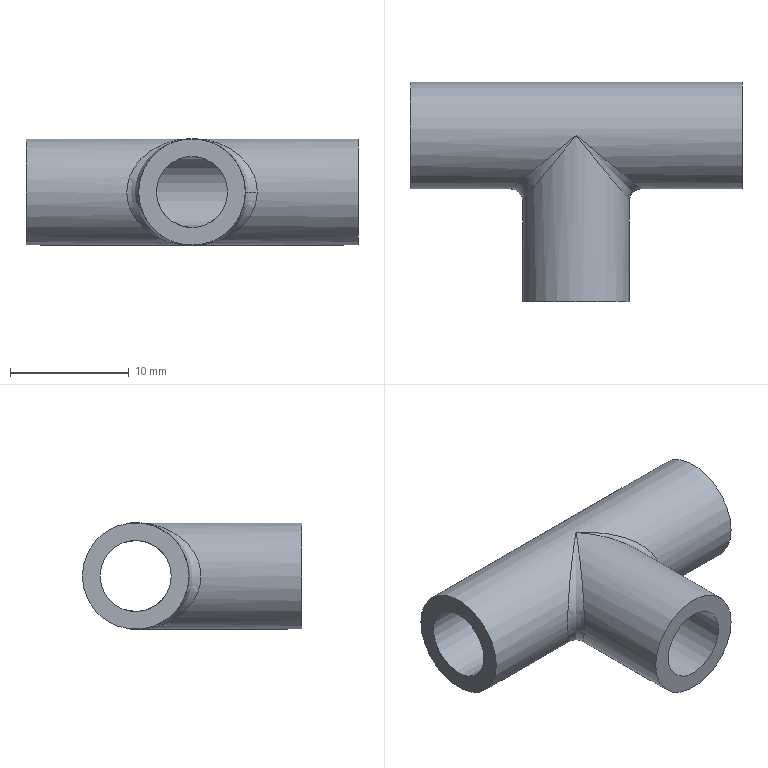Part | STEP file | 1-70.1 | 1 solid | 10 faces | box 28 x 18.5 x 9 mm | volume 1316 mm3 | cylinder 4 | plane 3 | spline 3 | commonest cylinder face diameters 6 x2 9 x2